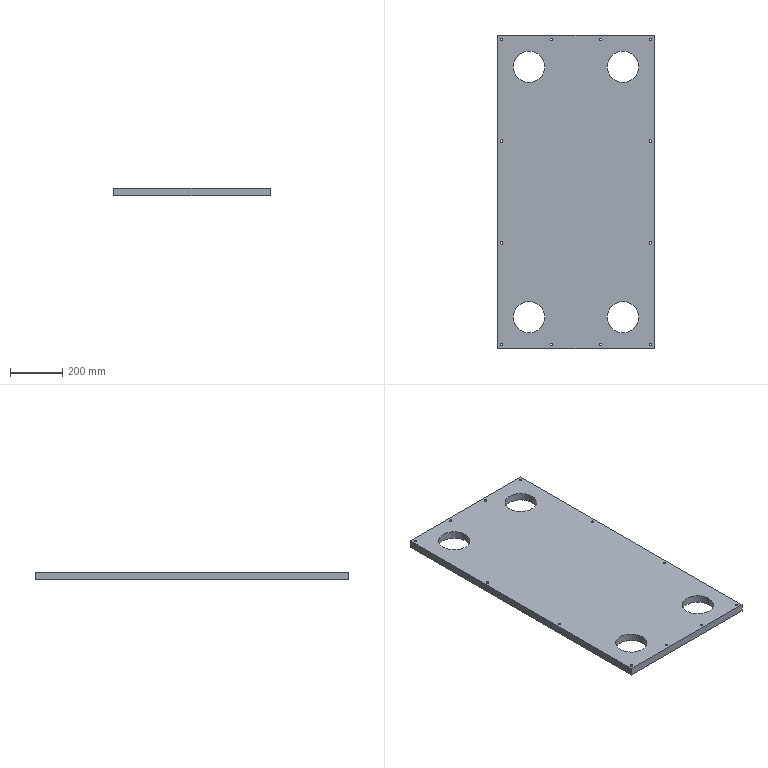Part | SolidWorks | features LPattern 8, ICE 3, Extrusion 1 | 1 solid | 74 faces | box 600 x 1200 x 30 mm | volume 20172146 mm3 | cylinder 56 | plane 18 | commonest cylinder face diameters 10 x24 20 x24 120 x8